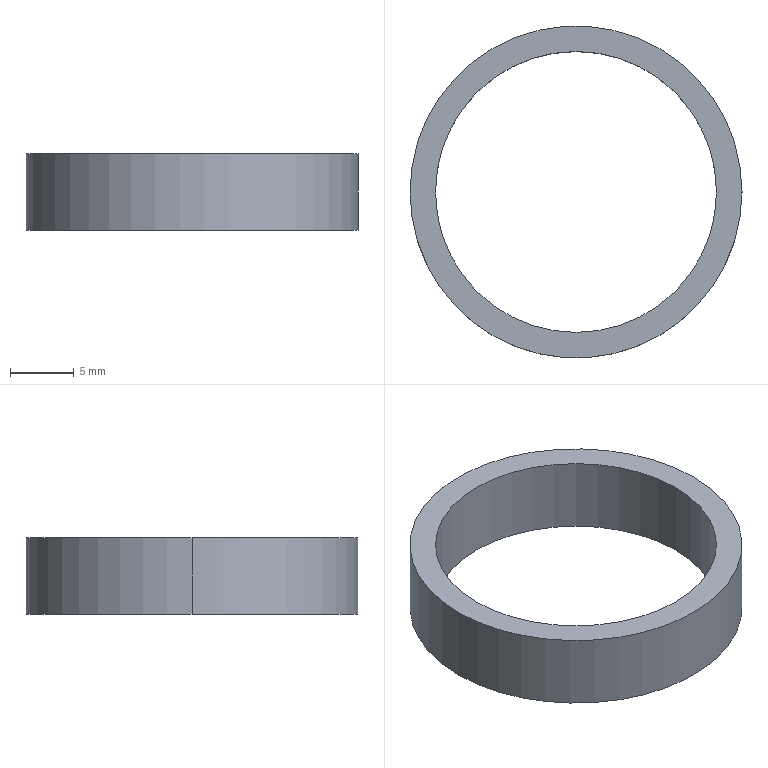Part | SolidWorks | features Extrusion 1 | 1 solid | 6 faces | box 26 x 26 x 6 mm | volume 904.779 mm3 | cylinder 4 | plane 2 | commonest cylinder face diameters 22 x2 26 x2
STEP:
#1=CARTESIAN_POINT('',(-11.,0.,6.));
#2=VERTEX_POINT('',#1);
#3=CARTESIAN_POINT('',(11.,0.,6.));
#4=VERTEX_POINT('',#3);
#5=CARTESIAN_POINT('',(0.,0.,6.));
#6=DIRECTION('',(0.,0.,1.));
#7=DIRECTION('',(1.,0.,0.));
#8=AXIS2_PLACEMENT_3D('',#5,#6,#7);
#9=CIRCLE('',#8,11.);
#10=EDGE_CURVE('',#2,#4,#9,.T.);
#11=ORIENTED_EDGE('',*,*,#10,.T.);
#12=CARTESIAN_POINT('',(11.,0.,0.));
#13=VERTEX_POINT('',#12);
#14=CARTESIAN_POINT('',(11.,0.,6.));
#15=DIRECTION('',(0.,0.,-1.));
#16=VECTOR('',#15,1000.);
#17=LINE('',#14,#16);
#18=EDGE_CURVE('',#4,#13,#17,.T.);
#19=ORIENTED_EDGE('',*,*,#18,.T.);
#20=CARTESIAN_POINT('',(-11.,0.,0.));
#21=VERTEX_POINT('',#20);
#22=CARTESIAN_POINT('',(0.,0.,0.));
#23=DIRECTION('',(0.,0.,1.));
#24=DIRECTION('',(1.,0.,0.));
#25=AXIS2_PLACEMENT_3D('',#22,#23,#24);
#26=CIRCLE('',#25,11.);
#27=EDGE_CURVE('',#21,#13,#26,.T.);
#28=ORIENTED_EDGE('',*,*,#27,.F.);
#29=CARTESIAN_POINT('',(-11.,0.,6.));
#30=DIRECTION('',(0.,0.,-1.));
#31=VECTOR('',#30,1000.);
#32=LINE('',#29,#31);
#33=EDGE_CURVE('',#2,#21,#32,.T.);
#34=ORIENTED_EDGE('',*,*,#33,.F.);
#35=EDGE_LOOP('',(#11,#19,#28,#34));
#36=FACE_OUTER_BOUND('',#35,.T.);
#37=CARTESIAN_POINT('',(0.,0.,6.));
#38=DIRECTION('',(0.,0.,-1.));
#39=DIRECTION('',(-1.,0.,0.));
#40=AXIS2_PLACEMENT_3D('',#37,#38,#39);
#41=CYLINDRICAL_SURFACE('',#40,11.);
#42=ADVANCED_FACE('',(#36),#41,.F.);
#43=CARTESIAN_POINT('',(13.,0.,6.));
#44=VERTEX_POINT('',#43);
#45=CARTESIAN_POINT('',(-13.,0.,6.));
#46=VERTEX_POINT('',#45);
#47=CARTESIAN_POINT('',(0.,0.,6.));
#48=DIRECTION('',(0.,0.,1.));
#49=DIRECTION('',(1.,0.,0.));
#50=AXIS2_PLACEMENT_3D('',#47,#48,#49);
#51=CIRCLE('',#50,13.);
#52=EDGE_CURVE('',#44,#46,#51,.T.);
#53=ORIENTED_EDGE('',*,*,#52,.F.);
#54=CARTESIAN_POINT('',(13.,0.,0.));
#55=VERTEX_POINT('',#54);
#56=CARTESIAN_POINT('',(13.,0.,6.));
#57=DIRECTION('',(0.,0.,-1.));
#58=VECTOR('',#57,1000.);
#59=LINE('',#56,#58);
#60=EDGE_CURVE('',#44,#55,#59,.T.);
#61=ORIENTED_EDGE('',*,*,#60,.T.);
#62=CARTESIAN_POINT('',(-13.,0.,0.));
#63=VERTEX_POINT('',#62);
#64=CARTESIAN_POINT('',(0.,0.,0.));
#65=DIRECTION('',(0.,0.,1.));
#66=DIRECTION('',(1.,0.,0.));
#67=AXIS2_PLACEMENT_3D('',#64,#65,#66);
#68=CIRCLE('',#67,13.);
#69=EDGE_CURVE('',#55,#63,#68,.T.);
#70=ORIENTED_EDGE('',*,*,#69,.T.);
#71=CARTESIAN_POINT('',(-13.,0.,6.));
#72=DIRECTION('',(0.,0.,-1.));
#73=VECTOR('',#72,1000.);
#74=LINE('',#71,#73);
#75=EDGE_CURVE('',#46,#63,#74,.T.);
#76=ORIENTED_EDGE('',*,*,#75,.F.);
#77=EDGE_LOOP('',(#53,#61,#70,#76));
#78=FACE_OUTER_BOUND('',#77,.T.);
#79=CARTESIAN_POINT('',(0.,0.,6.));
#80=DIRECTION('',(0.,0.,-1.));
#81=DIRECTION('',(-1.,0.,0.));
#82=AXIS2_PLACEMENT_3D('',#79,#80,#81);
#83=CYLINDRICAL_SURFACE('',#82,13.);
#84=ADVANCED_FACE('',(#78),#83,.T.);
#85=CARTESIAN_POINT('',(0.,0.,6.));
#86=DIRECTION('',(0.,0.,1.));
#87=DIRECTION('',(1.,0.,0.));
#88=AXIS2_PLACEMENT_3D('',#85,#86,#87);
#89=CIRCLE('',#88,13.);
#90=EDGE_CURVE('',#46,#44,#89,.T.);
#91=ORIENTED_EDGE('',*,*,#90,.T.);
#92=ORIENTED_EDGE('',*,*,#52,.T.);
#93=EDGE_LOOP('',(#91,#92));
#94=FACE_OUTER_BOUND('',#93,.T.);
#95=ORIENTED_EDGE('',*,*,#10,.F.);
#96=CARTESIAN_POINT('',(0.,0.,6.));
#97=DIRECTION('',(0.,0.,1.));
#98=DIRECTION('',(1.,0.,0.));
#99=AXIS2_PLACEMENT_3D('',#96,#97,#98);
#100=CIRCLE('',#99,11.);
#101=EDGE_CURVE('',#4,#2,#100,.T.);
#102=ORIENTED_EDGE('',*,*,#101,.F.);
#103=EDGE_LOOP('',(#95,#102));
#104=FACE_BOUND('',#103,.T.);
#105=CARTESIAN_POINT('',(0.,0.,6.));
#106=DIRECTION('',(0.,0.,1.));
#107=DIRECTION('',(1.,0.,0.));
#108=AXIS2_PLACEMENT_3D('',#105,#106,#107);
#109=PLANE('',#108);
#110=ADVANCED_FACE('',(#94,#104),#109,.T.);
#111=CARTESIAN_POINT('',(0.,0.,0.));
#112=DIRECTION('',(0.,0.,1.));
#113=DIRECTION('',(1.,0.,0.));
#114=AXIS2_PLACEMENT_3D('',#111,#112,#113);
#115=CIRCLE('',#114,13.);
#116=EDGE_CURVE('',#63,#55,#115,.T.);
#117=ORIENTED_EDGE('',*,*,#116,.F.);
#118=ORIENTED_EDGE('',*,*,#69,.F.);
#119=EDGE_LOOP('',(#117,#118));
#120=FACE_OUTER_BOUND('',#119,.T.);
#121=ORIENTED_EDGE('',*,*,#27,.T.);
#122=CARTESIAN_POINT('',(0.,0.,0.));
#123=DIRECTION('',(0.,0.,1.));
#124=DIRECTION('',(1.,0.,0.));
#125=AXIS2_PLACEMENT_3D('',#122,#123,#124);
#126=CIRCLE('',#125,11.);
#127=EDGE_CURVE('',#13,#21,#126,.T.);
#128=ORIENTED_EDGE('',*,*,#127,.T.);
#129=EDGE_LOOP('',(#121,#128));
#130=FACE_BOUND('',#129,.T.);
#131=CARTESIAN_POINT('',(0.,0.,0.));
#132=DIRECTION('',(0.,0.,1.));
#133=DIRECTION('',(1.,0.,0.));
#134=AXIS2_PLACEMENT_3D('',#131,#132,#133);
#135=PLANE('',#134);
#136=ADVANCED_FACE('',(#120,#130),#135,.F.);
#137=ORIENTED_EDGE('',*,*,#60,.F.);
#138=ORIENTED_EDGE('',*,*,#90,.F.);
#139=ORIENTED_EDGE('',*,*,#75,.T.);
#140=ORIENTED_EDGE('',*,*,#116,.T.);
#141=EDGE_LOOP('',(#137,#138,#139,#140));
#142=FACE_OUTER_BOUND('',#141,.T.);
#143=CARTESIAN_POINT('',(0.,0.,6.));
#144=DIRECTION('',(0.,0.,-1.));
#145=DIRECTION('',(-1.,0.,0.));
#146=AXIS2_PLACEMENT_3D('',#143,#144,#145);
#147=CYLINDRICAL_SURFACE('',#146,13.);
#148=ADVANCED_FACE('',(#142),#147,.T.);
#149=ORIENTED_EDGE('',*,*,#18,.F.);
#150=ORIENTED_EDGE('',*,*,#101,.T.);
#151=ORIENTED_EDGE('',*,*,#33,.T.);
#152=ORIENTED_EDGE('',*,*,#127,.F.);
#153=EDGE_LOOP('',(#149,#150,#151,#152));
#154=FACE_OUTER_BOUND('',#153,.T.);
#155=CARTESIAN_POINT('',(0.,0.,6.));
#156=DIRECTION('',(0.,0.,-1.));
#157=DIRECTION('',(-1.,0.,0.));
#158=AXIS2_PLACEMENT_3D('',#155,#156,#157);
#159=CYLINDRICAL_SURFACE('',#158,11.);
#160=ADVANCED_FACE('',(#154),#159,.F.);
#161=CLOSED_SHELL('',(#42,#84,#110,#136,#148,#160));
#162=MANIFOLD_SOLID_BREP('',#161);
#163=CARTESIAN_POINT('',(0.,0.,0.));
#164=DIRECTION('',(0.,0.,1.));
#165=DIRECTION('',(1.,0.,0.));
#166=AXIS2_PLACEMENT_3D('',#163,#164,#165);
#167=(LENGTH_UNIT()NAMED_UNIT(*)SI_UNIT(.MILLI.,.METRE.));
#168=UNCERTAINTY_MEASURE_WITH_UNIT(LENGTH_MEASURE(0.00001),#167,'','');
#169=(NAMED_UNIT(*)PLANE_ANGLE_UNIT()SI_UNIT($,.RADIAN.));
#170=(NAMED_UNIT(*)SI_UNIT($,.STERADIAN.)SOLID_ANGLE_UNIT());
#171=(GEOMETRIC_REPRESENTATION_CONTEXT(3)GLOBAL_UNCERTAINTY_ASSIGNED_CONTEXT((#168))GLOBAL_UNIT_ASSIGNED_CONTEXT((#167,#169,#170))REPRESENTATION_CONTEXT('',''));
#172=ADVANCED_BREP_SHAPE_REPRESENTATION('',(#162,#166),#171);